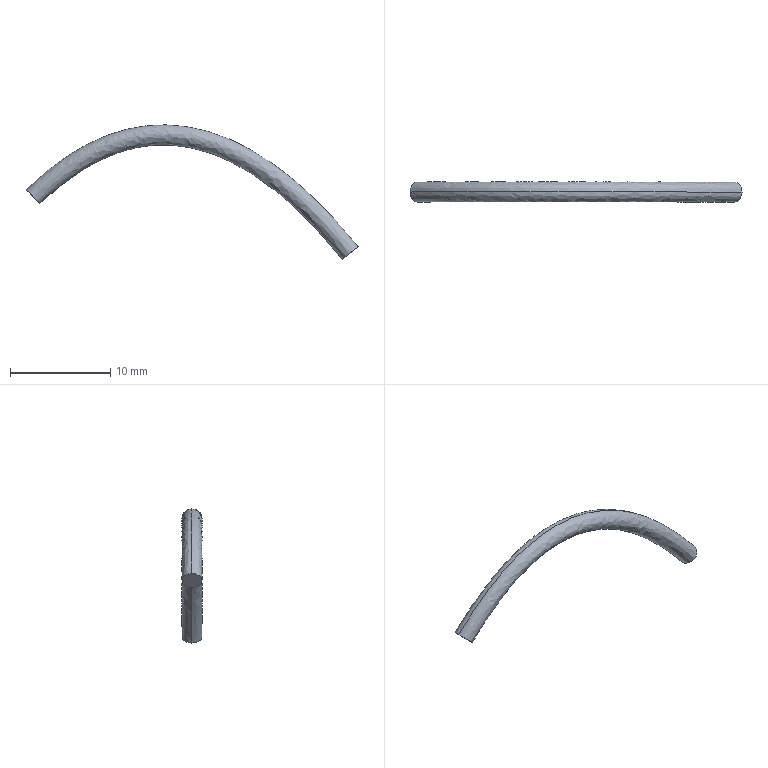Part | STEP file | YINGXIAN4_4_1 | 1 solid | 4 faces | box 33.17 x 2 x 13.408 mm | volume 118.062 mm3 | plane 2 | spline 2
STEP:
#1=CARTESIAN_POINT('',(0.,0.,0.));
#2=DIRECTION('',(0.,0.,1.));
#3=DIRECTION('',(1.,0.,0.));
#4=AXIS2_PLACEMENT_3D('',#1,#2,#3);
#5=CARTESIAN_POINT('',(0.6931,0.,-0.7208));
#6=VERTEX_POINT('',#5);
#7=CARTESIAN_POINT('',(-0.6931,0.,0.7208));
#8=VERTEX_POINT('',#7);
#9=CARTESIAN_POINT('',(0.6931,0.1194,-0.7208));
#10=CARTESIAN_POINT('',(0.6627,0.3767,-0.6892));
#11=CARTESIAN_POINT('',(0.5016,0.7326,-0.5216));
#12=CARTESIAN_POINT('',(0.2966,0.9207,-0.3085));
#13=CARTESIAN_POINT('',(0.1236,0.9898,-0.1286));
#14=CARTESIAN_POINT('',(0.,1.005,0.));
#15=CARTESIAN_POINT('',(-0.1236,0.9898,0.1286));
#16=CARTESIAN_POINT('',(-0.2966,0.9207,0.3085));
#17=CARTESIAN_POINT('',(-0.5016,0.7326,0.5216));
#18=CARTESIAN_POINT('',(-0.6627,0.3767,0.6892));
#19=CARTESIAN_POINT('',(-0.6931,0.1194,0.7208));
#20=B_SPLINE_CURVE_WITH_KNOTS('',3,(#5,#9,#10,#11,#12,#13,#14,#15,#16,#17,#18,#19,#7),.UNSPECIFIED.,.F.,.F.,(4,1,1,1,1,1,1,1,1,1,4),(0.,0.125,0.25,0.375,0.4375,0.5,0.5625,0.625,0.75,0.875,1.),.UNSPECIFIED.);
#21=EDGE_CURVE('',#6,#8,#20,.T.);
#22=ORIENTED_EDGE('',*,*,#21,.T.);
#23=CARTESIAN_POINT('',(-0.6931,0.,0.7208));
#24=CARTESIAN_POINT('',(-0.6931,-0.1194,0.7208));
#25=CARTESIAN_POINT('',(-0.6627,-0.3767,0.6892));
#26=CARTESIAN_POINT('',(-0.5016,-0.7326,0.5216));
#27=CARTESIAN_POINT('',(-0.2966,-0.9207,0.3085));
#28=CARTESIAN_POINT('',(-0.1236,-0.9898,0.1286));
#29=CARTESIAN_POINT('',(0.,-1.005,0.));
#30=CARTESIAN_POINT('',(0.1236,-0.9898,-0.1286));
#31=CARTESIAN_POINT('',(0.2966,-0.9207,-0.3085));
#32=CARTESIAN_POINT('',(0.5016,-0.7326,-0.5216));
#33=CARTESIAN_POINT('',(0.6627,-0.3767,-0.6892));
#34=CARTESIAN_POINT('',(0.6931,-0.1194,-0.7208));
#35=CARTESIAN_POINT('',(0.6931,0.,-0.7208));
#36=B_SPLINE_CURVE_WITH_KNOTS('',3,(#23,#24,#25,#26,#27,#28,#29,#30,#31,#32,#33,#34,#35),.UNSPECIFIED.,.F.,.F.,(4,1,1,1,1,1,1,1,1,1,4),(0.,0.125,0.25,0.375,0.4375,0.5,0.5625,0.625,0.75,0.875,1.),.UNSPECIFIED.);
#37=EDGE_CURVE('',#8,#6,#36,.T.);
#38=ORIENTED_EDGE('',*,*,#37,.T.);
#39=EDGE_LOOP('',(#22,#38));
#40=FACE_OUTER_BOUND('',#39,.F.);
#41=CARTESIAN_POINT('',(0.,0.,0.));
#42=DIRECTION('',(0.7208,0.,0.6931));
#43=DIRECTION('',(0.6931,0.,-0.7208));
#44=AXIS2_PLACEMENT_3D('',#41,#42,#43);
#45=PLANE('',#44);
#46=ADVANCED_FACE('',(#40),#45,.F.);
#47=ORIENTED_EDGE('',*,*,#21,.F.);
#48=CARTESIAN_POINT('',(30.923,0.,-6.249));
#49=VERTEX_POINT('',#48);
#50=CARTESIAN_POINT('',(0.6931,0.,-0.7208));
#51=CARTESIAN_POINT('',(2.159,0.,0.6885));
#52=CARTESIAN_POINT('',(4.382,0.,2.435));
#53=CARTESIAN_POINT('',(7.408,0.,4.024));
#54=CARTESIAN_POINT('',(9.717,0.,4.813));
#55=CARTESIAN_POINT('',(12.077,0.,5.194));
#56=CARTESIAN_POINT('',(14.439,0.,5.157));
#57=CARTESIAN_POINT('',(16.961,0.,4.657));
#58=CARTESIAN_POINT('',(20.428,0.,3.321));
#59=CARTESIAN_POINT('',(25.074,0.,0.2324));
#60=CARTESIAN_POINT('',(28.907,0.,-3.76));
#61=B_SPLINE_CURVE_WITH_KNOTS('',3,(#50,#51,#52,#53,#54,#55,#56,#57,#58,#59,#60,#48),.UNSPECIFIED.,.F.,.F.,(4,1,1,1,1,1,1,1,1,4),(0.,0.1483,0.2255,0.3091,0.3855,0.4682,0.551,0.6407,0.8132,1.),.UNSPECIFIED.);
#62=EDGE_CURVE('',#6,#49,#61,.T.);
#63=ORIENTED_EDGE('',*,*,#62,.T.);
#64=CARTESIAN_POINT('',(32.477,0.,-4.991));
#65=VERTEX_POINT('',#64);
#66=CARTESIAN_POINT('',(32.477,0.1194,-4.991));
#67=CARTESIAN_POINT('',(32.443,0.3767,-5.018));
#68=CARTESIAN_POINT('',(32.262,0.7326,-5.165));
#69=CARTESIAN_POINT('',(32.033,0.9207,-5.351));
#70=CARTESIAN_POINT('',(31.839,0.9898,-5.508));
#71=CARTESIAN_POINT('',(31.7,1.005,-5.62));
#72=CARTESIAN_POINT('',(31.561,0.9898,-5.732));
#73=CARTESIAN_POINT('',(31.367,0.9207,-5.889));
#74=CARTESIAN_POINT('',(31.138,0.7326,-6.075));
#75=CARTESIAN_POINT('',(30.957,0.3767,-6.222));
#76=CARTESIAN_POINT('',(30.923,0.1194,-6.249));
#77=CARTESIAN_POINT('',(30.923,0.,-6.249));
#78=B_SPLINE_CURVE_WITH_KNOTS('',3,(#64,#66,#67,#68,#69,#70,#71,#72,#73,#74,#75,#76,#77),.UNSPECIFIED.,.F.,.F.,(4,1,1,1,1,1,1,1,1,1,4),(0.,0.125,0.25,0.375,0.4375,0.5,0.5625,0.625,0.75,0.875,1.),.UNSPECIFIED.);
#79=EDGE_CURVE('',#65,#49,#78,.T.);
#80=ORIENTED_EDGE('',*,*,#79,.F.);
#81=CARTESIAN_POINT('',(-0.6931,0.,0.7208));
#82=CARTESIAN_POINT('',(0.8601,0.,2.214));
#83=CARTESIAN_POINT('',(3.251,0.,4.1));
#84=CARTESIAN_POINT('',(6.605,0.,5.865));
#85=CARTESIAN_POINT('',(9.22,0.,6.761));
#86=CARTESIAN_POINT('',(11.933,0.,7.2));
#87=CARTESIAN_POINT('',(14.657,0.,7.156));
#88=CARTESIAN_POINT('',(17.534,0.,6.584));
#89=CARTESIAN_POINT('',(21.407,0.,5.086));
#90=CARTESIAN_POINT('',(26.409,0.,1.742));
#91=CARTESIAN_POINT('',(30.398,0.,-2.424));
#92=CARTESIAN_POINT('',(32.477,0.,-4.991));
#93=B_SPLINE_CURVE_WITH_KNOTS('',3,(#81,#82,#83,#84,#85,#86,#87,#88,#89,#90,#91,#92),.UNSPECIFIED.,.F.,.F.,(4,1,1,1,1,1,1,1,1,4),(0.,0.1483,0.2255,0.3091,0.3855,0.4682,0.551,0.6407,0.8132,1.),.UNSPECIFIED.);
#94=EDGE_CURVE('',#8,#65,#93,.T.);
#95=ORIENTED_EDGE('',*,*,#94,.F.);
#96=EDGE_LOOP('',(#47,#63,#80,#95));
#97=FACE_OUTER_BOUND('',#96,.F.);
#98=CARTESIAN_POINT('',(0.4367,-0.03181,-0.9693));
#99=CARTESIAN_POINT('',(1.988,-0.03181,0.5542));
#100=CARTESIAN_POINT('',(4.298,-0.03181,2.391));
#101=CARTESIAN_POINT('',(7.408,-0.03181,4.025));
#102=CARTESIAN_POINT('',(9.717,-0.03181,4.814));
#103=CARTESIAN_POINT('',(12.077,-0.03181,5.195));
#104=CARTESIAN_POINT('',(14.439,-0.03181,5.157));
#105=CARTESIAN_POINT('',(16.961,-0.03181,4.658));
#106=CARTESIAN_POINT('',(20.429,-0.03181,3.321));
#107=CARTESIAN_POINT('',(25.147,-0.03181,0.1847));
#108=CARTESIAN_POINT('',(29.057,-0.03181,-3.916));
#109=CARTESIAN_POINT('',(31.15,-0.03181,-6.53));
#110=CARTESIAN_POINT('',(0.4397,0.09633,-0.9723));
#111=CARTESIAN_POINT('',(1.991,0.09633,0.551));
#112=CARTESIAN_POINT('',(4.3,0.09633,2.388));
#113=CARTESIAN_POINT('',(7.41,0.09633,4.021));
#114=CARTESIAN_POINT('',(9.718,0.09633,4.81));
#115=CARTESIAN_POINT('',(12.077,0.09633,5.19));
#116=CARTESIAN_POINT('',(14.439,0.09633,5.153));
#117=CARTESIAN_POINT('',(16.959,0.09633,4.654));
#118=CARTESIAN_POINT('',(20.427,0.09633,3.317));
#119=CARTESIAN_POINT('',(25.144,0.09633,0.1816));
#120=CARTESIAN_POINT('',(29.054,0.09633,-3.919));
#121=CARTESIAN_POINT('',(31.146,0.09633,-6.533));
#122=CARTESIAN_POINT('',(0.4112,0.3661,-0.9433));
#123=CARTESIAN_POINT('',(1.964,0.3661,0.5818));
#124=CARTESIAN_POINT('',(4.277,0.3661,2.422));
#125=CARTESIAN_POINT('',(7.393,0.3661,4.058));
#126=CARTESIAN_POINT('',(9.708,0.3661,4.849));
#127=CARTESIAN_POINT('',(12.074,0.3661,5.231));
#128=CARTESIAN_POINT('',(14.443,0.3661,5.194));
#129=CARTESIAN_POINT('',(16.971,0.3661,4.693));
#130=CARTESIAN_POINT('',(20.447,0.3661,3.353));
#131=CARTESIAN_POINT('',(25.171,0.3661,0.2122));
#132=CARTESIAN_POINT('',(29.084,0.3661,-3.892));
#133=CARTESIAN_POINT('',(31.178,0.3661,-6.507));
#134=CARTESIAN_POINT('',(0.2435,0.7326,-0.7725));
#135=CARTESIAN_POINT('',(1.807,0.7326,0.7631));
#136=CARTESIAN_POINT('',(4.14,0.7326,2.62));
#137=CARTESIAN_POINT('',(7.297,0.7326,4.279));
#138=CARTESIAN_POINT('',(9.649,0.7326,5.082));
#139=CARTESIAN_POINT('',(12.057,0.7326,5.471));
#140=CARTESIAN_POINT('',(14.469,0.7326,5.433));
#141=CARTESIAN_POINT('',(17.04,0.7326,4.923));
#142=CARTESIAN_POINT('',(20.564,0.7326,3.565));
#143=CARTESIAN_POINT('',(25.331,0.7326,0.3923));
#144=CARTESIAN_POINT('',(29.263,0.7326,-3.733));
#145=CARTESIAN_POINT('',(31.365,0.7326,-6.358));
#146=CARTESIAN_POINT('',(0.03628,0.9207,-0.5615));
#147=CARTESIAN_POINT('',(1.613,0.9207,0.9871));
#148=CARTESIAN_POINT('',(3.972,0.9207,2.866));
#149=CARTESIAN_POINT('',(7.178,0.9207,4.551));
#150=CARTESIAN_POINT('',(9.575,0.9207,5.37));
#151=CARTESIAN_POINT('',(12.036,0.9207,5.768));
#152=CARTESIAN_POINT('',(14.501,0.9207,5.728));
#153=CARTESIAN_POINT('',(17.124,0.9207,5.208));
#154=CARTESIAN_POINT('',(20.708,0.9207,3.826));
#155=CARTESIAN_POINT('',(25.53,0.9207,0.6148));
#156=CARTESIAN_POINT('',(29.484,0.9207,-3.536));
#157=CARTESIAN_POINT('',(31.596,0.9207,-6.173));
#158=CARTESIAN_POINT('',(-0.1386,0.9898,-0.3834));
#159=CARTESIAN_POINT('',(1.45,0.9897,1.176));
#160=CARTESIAN_POINT('',(3.829,0.9898,3.073));
#161=CARTESIAN_POINT('',(7.078,0.9898,4.78));
#162=CARTESIAN_POINT('',(9.513,0.9898,5.613));
#163=CARTESIAN_POINT('',(12.018,0.9898,6.018));
#164=CARTESIAN_POINT('',(14.529,0.9897,5.978));
#165=CARTESIAN_POINT('',(17.196,0.9897,5.449));
#166=CARTESIAN_POINT('',(20.83,0.9898,4.046));
#167=CARTESIAN_POINT('',(25.697,0.9898,0.8026));
#168=CARTESIAN_POINT('',(29.671,0.9897,-3.37));
#169=CARTESIAN_POINT('',(31.791,0.9898,-6.017));
#170=CARTESIAN_POINT('',(-0.2636,1.005,-0.2562));
#171=CARTESIAN_POINT('',(1.333,1.005,1.311));
#172=CARTESIAN_POINT('',(3.728,1.005,3.221));
#173=CARTESIAN_POINT('',(7.007,1.005,4.945));
#174=CARTESIAN_POINT('',(9.469,1.005,5.787));
#175=CARTESIAN_POINT('',(12.005,1.005,6.197));
#176=CARTESIAN_POINT('',(14.548,1.005,6.156));
#177=CARTESIAN_POINT('',(17.247,1.005,5.621));
#178=CARTESIAN_POINT('',(20.918,1.005,4.204));
#179=CARTESIAN_POINT('',(25.817,1.005,0.9369));
#180=CARTESIAN_POINT('',(29.805,1.005,-3.251));
#181=CARTESIAN_POINT('',(31.93,1.005,-5.905));
#182=CARTESIAN_POINT('',(-0.3886,0.9898,-0.1289));
#183=CARTESIAN_POINT('',(1.216,0.9897,1.447));
#184=CARTESIAN_POINT('',(3.626,0.9898,3.369));
#185=CARTESIAN_POINT('',(6.935,0.9898,5.109));
#186=CARTESIAN_POINT('',(9.425,0.9898,5.961));
#187=CARTESIAN_POINT('',(11.992,0.9898,6.376));
#188=CARTESIAN_POINT('',(14.568,0.9897,6.334));
#189=CARTESIAN_POINT('',(17.298,0.9897,5.793));
#190=CARTESIAN_POINT('',(21.005,0.9898,4.361));
#191=CARTESIAN_POINT('',(25.936,0.9898,1.071));
#192=CARTESIAN_POINT('',(29.938,0.9897,-3.133));
#193=CARTESIAN_POINT('',(32.069,0.9898,-5.794));
#194=CARTESIAN_POINT('',(-0.5635,0.9207,0.0492));
#195=CARTESIAN_POINT('',(1.052,0.9207,1.636));
#196=CARTESIAN_POINT('',(3.484,0.9207,3.576));
#197=CARTESIAN_POINT('',(6.835,0.9207,5.338));
#198=CARTESIAN_POINT('',(9.363,0.9207,6.204));
#199=CARTESIAN_POINT('',(11.974,0.9207,6.626));
#200=CARTESIAN_POINT('',(14.595,0.9207,6.584));
#201=CARTESIAN_POINT('',(17.37,0.9207,6.033));
#202=CARTESIAN_POINT('',(21.127,0.9207,4.581));
#203=CARTESIAN_POINT('',(26.104,0.9207,1.259));
#204=CARTESIAN_POINT('',(30.125,0.9207,-2.967));
#205=CARTESIAN_POINT('',(32.264,0.9207,-5.638));
#206=CARTESIAN_POINT('',(-0.7707,0.7326,0.2602));
#207=CARTESIAN_POINT('',(0.8581,0.7326,1.86));
#208=CARTESIAN_POINT('',(3.315,0.7326,3.821));
#209=CARTESIAN_POINT('',(6.716,0.7326,5.611));
#210=CARTESIAN_POINT('',(9.289,0.7326,6.492));
#211=CARTESIAN_POINT('',(11.953,0.7326,6.922));
#212=CARTESIAN_POINT('',(14.627,0.7326,6.88));
#213=CARTESIAN_POINT('',(17.454,0.7326,6.318));
#214=CARTESIAN_POINT('',(21.272,0.7326,4.842));
#215=CARTESIAN_POINT('',(26.302,0.7326,1.482));
#216=CARTESIAN_POINT('',(30.346,0.7326,-2.77));
#217=CARTESIAN_POINT('',(32.495,0.7326,-5.453));
#218=CARTESIAN_POINT('',(-0.9383,0.3663,0.4309));
#219=CARTESIAN_POINT('',(0.7012,0.3663,2.041));
#220=CARTESIAN_POINT('',(3.178,0.3663,4.02));
#221=CARTESIAN_POINT('',(6.62,0.3663,5.831));
#222=CARTESIAN_POINT('',(9.23,0.3663,6.725));
#223=CARTESIAN_POINT('',(11.936,0.3663,7.162));
#224=CARTESIAN_POINT('',(14.653,0.3663,7.119));
#225=CARTESIAN_POINT('',(17.523,0.3663,6.548));
#226=CARTESIAN_POINT('',(21.389,0.3663,5.054));
#227=CARTESIAN_POINT('',(26.462,0.3663,1.662));
#228=CARTESIAN_POINT('',(30.525,0.3663,-2.611));
#229=CARTESIAN_POINT('',(32.682,0.3663,-5.304));
#230=CARTESIAN_POINT('',(-0.9668,0.09668,0.4599));
#231=CARTESIAN_POINT('',(0.6746,0.09668,2.072));
#232=CARTESIAN_POINT('',(3.155,0.09668,4.054));
#233=CARTESIAN_POINT('',(6.604,0.09668,5.868));
#234=CARTESIAN_POINT('',(9.22,0.09668,6.764));
#235=CARTESIAN_POINT('',(11.933,0.09668,7.203));
#236=CARTESIAN_POINT('',(14.658,0.09668,7.159));
#237=CARTESIAN_POINT('',(17.535,0.09668,6.588));
#238=CARTESIAN_POINT('',(21.409,0.09668,5.09));
#239=CARTESIAN_POINT('',(26.49,0.09668,1.692));
#240=CARTESIAN_POINT('',(30.556,0.09668,-2.584));
#241=CARTESIAN_POINT('',(32.713,0.09668,-5.278));
#242=CARTESIAN_POINT('',(-0.9639,-0.03133,0.457));
#243=CARTESIAN_POINT('',(0.6773,-0.03133,2.069));
#244=CARTESIAN_POINT('',(3.158,-0.03133,4.05));
#245=CARTESIAN_POINT('',(6.605,-0.03133,5.864));
#246=CARTESIAN_POINT('',(9.221,-0.03133,6.76));
#247=CARTESIAN_POINT('',(11.933,-0.03133,7.199));
#248=CARTESIAN_POINT('',(14.657,-0.03133,7.155));
#249=CARTESIAN_POINT('',(17.533,-0.03133,6.584));
#250=CARTESIAN_POINT('',(21.407,-0.03133,5.086));
#251=CARTESIAN_POINT('',(26.487,-0.03133,1.689));
#252=CARTESIAN_POINT('',(30.553,-0.03133,-2.586));
#253=CARTESIAN_POINT('',(32.71,-0.03133,-5.281));
#254=B_SPLINE_SURFACE_WITH_KNOTS('',3,3,((#98,#99,#100,#101,#102,#103,#104,#105,#106,#107,#108,#109),(#110,#111,#112,#113,#114,#115,#116,#117,#118,#119,#120,#121),(#122,#123,#124,#125,#126,#127,#128,#129,#130,#131,#132,#133),(#134,#135,#136,#137,#138,#139,#140,#141,#142,#143,#144,#145),(#146,#147,#148,#149,#150,#151,#152,#153,#154,#155,#156,#157),(#158,#159,#160,#161,#162,#163,#164,#165,#166,#167,#168,#169),(#170,#171,#172,#173,#174,#175,#176,#177,#178,#179,#180,#181),(#182,#183,#184,#185,#186,#187,#188,#189,#190,#191,#192,#193),(#194,#195,#196,#197,#198,#199,#200,#201,#202,#203,#204,#205),(#206,#207,#208,#209,#210,#211,#212,#213,#214,#215,#216,#217),(#218,#219,#220,#221,#222,#223,#224,#225,#226,#227,#228,#229),(#230,#231,#232,#233,#234,#235,#236,#237,#238,#239,#240,#241),(#242,#243,#244,#245,#246,#247,#248,#249,#250,#251,#252,#253)),.UNSPECIFIED.,.F.,.F.,.F.,(4,1,1,1,1,1,1,1,1,1,4),(4,1,1,1,1,1,1,1,1,4),(0.02112,0.2819,0.5213,0.7606,0.8803,1.,1.12,1.239,1.479,1.718,1.979),(-0.008638,0.1483,0.2255,0.3091,0.3855,0.4682,0.551,0.6407,0.8132,1.007),.UNSPECIFIED.);
#255=ADVANCED_FACE('',(#97),#254,.T.);
#256=ORIENTED_EDGE('',*,*,#37,.F.);
#257=ORIENTED_EDGE('',*,*,#94,.T.);
#258=CARTESIAN_POINT('',(30.923,0.,-6.249));
#259=CARTESIAN_POINT('',(30.923,-0.1194,-6.249));
#260=CARTESIAN_POINT('',(30.957,-0.3767,-6.222));
#261=CARTESIAN_POINT('',(31.138,-0.7326,-6.075));
#262=CARTESIAN_POINT('',(31.367,-0.9207,-5.889));
#263=CARTESIAN_POINT('',(31.561,-0.9898,-5.732));
#264=CARTESIAN_POINT('',(31.7,-1.005,-5.62));
#265=CARTESIAN_POINT('',(31.839,-0.9898,-5.508));
#266=CARTESIAN_POINT('',(32.033,-0.9207,-5.351));
#267=CARTESIAN_POINT('',(32.262,-0.7326,-5.165));
#268=CARTESIAN_POINT('',(32.443,-0.3767,-5.018));
#269=CARTESIAN_POINT('',(32.477,-0.1194,-4.991));
#270=CARTESIAN_POINT('',(32.477,0.,-4.991));
#271=B_SPLINE_CURVE_WITH_KNOTS('',3,(#258,#259,#260,#261,#262,#263,#264,#265,#266,#267,#268,#269,#270),.UNSPECIFIED.,.F.,.F.,(4,1,1,1,1,1,1,1,1,1,4),(0.,0.125,0.25,0.375,0.4375,0.5,0.5625,0.625,0.75,0.875,1.),.UNSPECIFIED.);
#272=EDGE_CURVE('',#49,#65,#271,.T.);
#273=ORIENTED_EDGE('',*,*,#272,.F.);
#274=ORIENTED_EDGE('',*,*,#62,.F.);
#275=EDGE_LOOP('',(#256,#257,#273,#274));
#276=FACE_OUTER_BOUND('',#275,.F.);
#277=CARTESIAN_POINT('',(-0.9639,0.03181,0.4569));
#278=CARTESIAN_POINT('',(0.6773,0.03181,2.069));
#279=CARTESIAN_POINT('',(3.158,0.03181,4.05));
#280=CARTESIAN_POINT('',(6.605,0.03181,5.864));
#281=CARTESIAN_POINT('',(9.221,0.03181,6.76));
#282=CARTESIAN_POINT('',(11.933,0.03181,7.199));
#283=CARTESIAN_POINT('',(14.657,0.03181,7.155));
#284=CARTESIAN_POINT('',(17.533,0.03181,6.584));
#285=CARTESIAN_POINT('',(21.407,0.03181,5.086));
#286=CARTESIAN_POINT('',(26.487,0.03181,1.689));
#287=CARTESIAN_POINT('',(30.553,0.03181,-2.587));
#288=CARTESIAN_POINT('',(32.71,0.03181,-5.281));
#289=CARTESIAN_POINT('',(-0.9669,-0.09633,0.46));
#290=CARTESIAN_POINT('',(0.6745,-0.09633,2.072));
#291=CARTESIAN_POINT('',(3.155,-0.09633,4.054));
#292=CARTESIAN_POINT('',(6.604,-0.09633,5.868));
#293=CARTESIAN_POINT('',(9.22,-0.09633,6.764));
#294=CARTESIAN_POINT('',(11.933,-0.09633,7.203));
#295=CARTESIAN_POINT('',(14.658,-0.09633,7.159));
#296=CARTESIAN_POINT('',(17.535,-0.09633,6.588));
#297=CARTESIAN_POINT('',(21.409,-0.09633,5.09));
#298=CARTESIAN_POINT('',(26.49,-0.09633,1.692));
#299=CARTESIAN_POINT('',(30.556,-0.09633,-2.584));
#300=CARTESIAN_POINT('',(32.713,-0.09633,-5.278));
#301=CARTESIAN_POINT('',(-0.9384,-0.3661,0.431));
#302=CARTESIAN_POINT('',(0.7012,-0.3661,2.041));
#303=CARTESIAN_POINT('',(3.178,-0.3661,4.02));
#304=CARTESIAN_POINT('',(6.62,-0.3661,5.831));
#305=CARTESIAN_POINT('',(9.23,-0.3661,6.725));
#306=CARTESIAN_POINT('',(11.936,-0.3661,7.162));
#307=CARTESIAN_POINT('',(14.653,-0.3661,7.119));
#308=CARTESIAN_POINT('',(17.523,-0.3661,6.548));
#309=CARTESIAN_POINT('',(21.389,-0.3661,5.054));
#310=CARTESIAN_POINT('',(26.462,-0.3661,1.662));
#311=CARTESIAN_POINT('',(30.526,-0.3661,-2.611));
#312=CARTESIAN_POINT('',(32.682,-0.3661,-5.304));
#313=CARTESIAN_POINT('',(-0.7707,-0.7326,0.2602));
#314=CARTESIAN_POINT('',(0.8581,-0.7326,1.86));
#315=CARTESIAN_POINT('',(3.315,-0.7326,3.821));
#316=CARTESIAN_POINT('',(6.716,-0.7326,5.611));
#317=CARTESIAN_POINT('',(9.289,-0.7326,6.492));
#318=CARTESIAN_POINT('',(11.953,-0.7326,6.922));
#319=CARTESIAN_POINT('',(14.627,-0.7326,6.88));
#320=CARTESIAN_POINT('',(17.454,-0.7326,6.318));
#321=CARTESIAN_POINT('',(21.272,-0.7326,4.842));
#322=CARTESIAN_POINT('',(26.302,-0.7326,1.482));
#323=CARTESIAN_POINT('',(30.346,-0.7326,-2.77));
#324=CARTESIAN_POINT('',(32.495,-0.7326,-5.453));
#325=CARTESIAN_POINT('',(-0.5635,-0.9207,0.0492));
#326=CARTESIAN_POINT('',(1.052,-0.9207,1.636));
#327=CARTESIAN_POINT('',(3.484,-0.9207,3.576));
#328=CARTESIAN_POINT('',(6.835,-0.9207,5.338));
#329=CARTESIAN_POINT('',(9.363,-0.9207,6.204));
#330=CARTESIAN_POINT('',(11.974,-0.9207,6.626));
#331=CARTESIAN_POINT('',(14.595,-0.9207,6.584));
#332=CARTESIAN_POINT('',(17.37,-0.9207,6.033));
#333=CARTESIAN_POINT('',(21.127,-0.9207,4.581));
#334=CARTESIAN_POINT('',(26.104,-0.9207,1.259));
#335=CARTESIAN_POINT('',(30.125,-0.9207,-2.967));
#336=CARTESIAN_POINT('',(32.264,-0.9207,-5.638));
#337=CARTESIAN_POINT('',(-0.3886,-0.9898,-0.1289));
#338=CARTESIAN_POINT('',(1.216,-0.9897,1.447));
#339=CARTESIAN_POINT('',(3.626,-0.9898,3.369));
#340=CARTESIAN_POINT('',(6.935,-0.9898,5.109));
#341=CARTESIAN_POINT('',(9.425,-0.9898,5.961));
#342=CARTESIAN_POINT('',(11.992,-0.9898,6.376));
#343=CARTESIAN_POINT('',(14.568,-0.9897,6.334));
#344=CARTESIAN_POINT('',(17.298,-0.9897,5.793));
#345=CARTESIAN_POINT('',(21.005,-0.9898,4.361));
#346=CARTESIAN_POINT('',(25.936,-0.9898,1.071));
#347=CARTESIAN_POINT('',(29.938,-0.9897,-3.133));
#348=CARTESIAN_POINT('',(32.069,-0.9898,-5.794));
#349=CARTESIAN_POINT('',(-0.2636,-1.005,-0.2562));
#350=CARTESIAN_POINT('',(1.333,-1.005,1.311));
#351=CARTESIAN_POINT('',(3.728,-1.005,3.221));
#352=CARTESIAN_POINT('',(7.007,-1.005,4.945));
#353=CARTESIAN_POINT('',(9.469,-1.005,5.787));
#354=CARTESIAN_POINT('',(12.005,-1.005,6.197));
#355=CARTESIAN_POINT('',(14.548,-1.005,6.156));
#356=CARTESIAN_POINT('',(17.247,-1.005,5.621));
#357=CARTESIAN_POINT('',(20.918,-1.005,4.204));
#358=CARTESIAN_POINT('',(25.817,-1.005,0.9369));
#359=CARTESIAN_POINT('',(29.805,-1.005,-3.251));
#360=CARTESIAN_POINT('',(31.93,-1.005,-5.905));
#361=CARTESIAN_POINT('',(-0.1386,-0.9898,-0.3834));
#362=CARTESIAN_POINT('',(1.45,-0.9897,1.176));
#363=CARTESIAN_POINT('',(3.829,-0.9898,3.073));
#364=CARTESIAN_POINT('',(7.078,-0.9898,4.78));
#365=CARTESIAN_POINT('',(9.513,-0.9898,5.613));
#366=CARTESIAN_POINT('',(12.018,-0.9898,6.018));
#367=CARTESIAN_POINT('',(14.529,-0.9897,5.978));
#368=CARTESIAN_POINT('',(17.196,-0.9897,5.449));
#369=CARTESIAN_POINT('',(20.83,-0.9898,4.046));
#370=CARTESIAN_POINT('',(25.697,-0.9898,0.8026));
#371=CARTESIAN_POINT('',(29.671,-0.9897,-3.37));
#372=CARTESIAN_POINT('',(31.791,-0.9898,-6.017));
#373=CARTESIAN_POINT('',(0.03628,-0.9207,-0.5615));
#374=CARTESIAN_POINT('',(1.613,-0.9207,0.9871));
#375=CARTESIAN_POINT('',(3.972,-0.9207,2.866));
#376=CARTESIAN_POINT('',(7.178,-0.9207,4.551));
#377=CARTESIAN_POINT('',(9.575,-0.9207,5.37));
#378=CARTESIAN_POINT('',(12.036,-0.9207,5.768));
#379=CARTESIAN_POINT('',(14.501,-0.9207,5.728));
#380=CARTESIAN_POINT('',(17.124,-0.9207,5.208));
#381=CARTESIAN_POINT('',(20.708,-0.9207,3.826));
#382=CARTESIAN_POINT('',(25.53,-0.9207,0.6148));
#383=CARTESIAN_POINT('',(29.484,-0.9207,-3.536));
#384=CARTESIAN_POINT('',(31.596,-0.9207,-6.173));
#385=CARTESIAN_POINT('',(0.2435,-0.7326,-0.7725));
#386=CARTESIAN_POINT('',(1.807,-0.7326,0.7631));
#387=CARTESIAN_POINT('',(4.14,-0.7326,2.62));
#388=CARTESIAN_POINT('',(7.297,-0.7326,4.279));
#389=CARTESIAN_POINT('',(9.649,-0.7326,5.082));
#390=CARTESIAN_POINT('',(12.057,-0.7326,5.471));
#391=CARTESIAN_POINT('',(14.469,-0.7326,5.433));
#392=CARTESIAN_POINT('',(17.04,-0.7326,4.923));
#393=CARTESIAN_POINT('',(20.564,-0.7326,3.565));
#394=CARTESIAN_POINT('',(25.331,-0.7326,0.3923));
#395=CARTESIAN_POINT('',(29.263,-0.7326,-3.733));
#396=CARTESIAN_POINT('',(31.365,-0.7326,-6.358));
#397=CARTESIAN_POINT('',(0.4111,-0.3663,-0.9432));
#398=CARTESIAN_POINT('',(1.964,-0.3663,0.5819));
#399=CARTESIAN_POINT('',(4.277,-0.3663,2.422));
#400=CARTESIAN_POINT('',(7.393,-0.3663,4.059));
#401=CARTESIAN_POINT('',(9.708,-0.3663,4.849));
#402=CARTESIAN_POINT('',(12.074,-0.3663,5.231));
#403=CARTESIAN_POINT('',(14.443,-0.3663,5.194));
#404=CARTESIAN_POINT('',(16.971,-0.3663,4.693));
#405=CARTESIAN_POINT('',(20.447,-0.3663,3.353));
#406=CARTESIAN_POINT('',(25.171,-0.3663,0.2122));
#407=CARTESIAN_POINT('',(29.084,-0.3663,-3.892));
#408=CARTESIAN_POINT('',(31.178,-0.3663,-6.507));
#409=CARTESIAN_POINT('',(0.4396,-0.09668,-0.9723));
#410=CARTESIAN_POINT('',(1.991,-0.09668,0.551));
#411=CARTESIAN_POINT('',(4.3,-0.09668,2.388));
#412=CARTESIAN_POINT('',(7.41,-0.09668,4.021));
#413=CARTESIAN_POINT('',(9.718,-0.09668,4.81));
#414=CARTESIAN_POINT('',(12.077,-0.09668,5.19));
#415=CARTESIAN_POINT('',(14.439,-0.09668,5.153));
#416=CARTESIAN_POINT('',(16.959,-0.09668,4.654));
#417=CARTESIAN_POINT('',(20.427,-0.09668,3.318));
#418=CARTESIAN_POINT('',(25.144,-0.09668,0.1816));
#419=CARTESIAN_POINT('',(29.054,-0.09668,-3.919));
#420=CARTESIAN_POINT('',(31.146,-0.09668,-6.533));
#421=CARTESIAN_POINT('',(0.4367,0.03133,-0.9693));
#422=CARTESIAN_POINT('',(1.988,0.03133,0.5542));
#423=CARTESIAN_POINT('',(4.298,0.03133,2.391));
#424=CARTESIAN_POINT('',(7.408,0.03133,4.025));
#425=CARTESIAN_POINT('',(9.717,0.03133,4.814));
#426=CARTESIAN_POINT('',(12.077,0.03133,5.195));
#427=CARTESIAN_POINT('',(14.439,0.03133,5.157));
#428=CARTESIAN_POINT('',(16.961,0.03133,4.658));
#429=CARTESIAN_POINT('',(20.429,0.03133,3.321));
#430=CARTESIAN_POINT('',(25.147,0.03133,0.1847));
#431=CARTESIAN_POINT('',(29.057,0.03133,-3.916));
#432=CARTESIAN_POINT('',(31.15,0.03133,-6.53));
#433=B_SPLINE_SURFACE_WITH_KNOTS('',3,3,((#277,#278,#279,#280,#281,#282,#283,#284,#285,#286,#287,#288),(#289,#290,#291,#292,#293,#294,#295,#296,#297,#298,#299,#300),(#301,#302,#303,#304,#305,#306,#307,#308,#309,#310,#311,#312),(#313,#314,#315,#316,#317,#318,#319,#320,#321,#322,#323,#324),(#325,#326,#327,#328,#329,#330,#331,#332,#333,#334,#335,#336),(#337,#338,#339,#340,#341,#342,#343,#344,#345,#346,#347,#348),(#349,#350,#351,#352,#353,#354,#355,#356,#357,#358,#359,#360),(#361,#362,#363,#364,#365,#366,#367,#368,#369,#370,#371,#372),(#373,#374,#375,#376,#377,#378,#379,#380,#381,#382,#383,#384),(#385,#386,#387,#388,#389,#390,#391,#392,#393,#394,#395,#396),(#397,#398,#399,#400,#401,#402,#403,#404,#405,#406,#407,#408),(#409,#410,#411,#412,#413,#414,#415,#416,#417,#418,#419,#420),(#421,#422,#423,#424,#425,#426,#427,#428,#429,#430,#431,#432)),.UNSPECIFIED.,.F.,.F.,.F.,(4,1,1,1,1,1,1,1,1,1,4),(4,1,1,1,1,1,1,1,1,4),(0.02112,0.2819,0.5213,0.7606,0.8803,1.,1.12,1.239,1.479,1.718,1.979),(-0.008638,0.1483,0.2255,0.3091,0.3855,0.4682,0.551,0.6407,0.8132,1.007),.UNSPECIFIED.);
#434=ADVANCED_FACE('',(#276),#433,.T.);
#435=ORIENTED_EDGE('',*,*,#79,.T.);
#436=ORIENTED_EDGE('',*,*,#272,.T.);
#437=EDGE_LOOP('',(#435,#436));
#438=FACE_OUTER_BOUND('',#437,.F.);
#439=CARTESIAN_POINT('',(31.7,0.,-5.62));
#440=DIRECTION('',(0.6294,0.,-0.7771));
#441=DIRECTION('',(-0.7771,0.,-0.6294));
#442=AXIS2_PLACEMENT_3D('',#439,#440,#441);
#443=PLANE('',#442);
#444=ADVANCED_FACE('',(#438),#443,.T.);
#445=CLOSED_SHELL('',(#46,#255,#434,#444));
#446=MANIFOLD_SOLID_BREP('',#445);
#447=(LENGTH_UNIT()NAMED_UNIT(*)SI_UNIT(.MILLI.,.METRE.));
#448=UNCERTAINTY_MEASURE_WITH_UNIT(LENGTH_MEASURE(0.003595),#447,'','');
#449=(NAMED_UNIT(*)PLANE_ANGLE_UNIT()SI_UNIT($,.RADIAN.));
#450=PLANE_ANGLE_MEASURE_WITH_UNIT(PLANE_ANGLE_MEASURE(0.01745),#449);
#451=(CONVERSION_BASED_UNIT('DEGREE',#450)NAMED_UNIT(*)PLANE_ANGLE_UNIT());
#452=(NAMED_UNIT(*)SI_UNIT($,.STERADIAN.)SOLID_ANGLE_UNIT());
#453=(GEOMETRIC_REPRESENTATION_CONTEXT(3)GLOBAL_UNCERTAINTY_ASSIGNED_CONTEXT((#448))GLOBAL_UNIT_ASSIGNED_CONTEXT((#447,#451,#452))REPRESENTATION_CONTEXT('',''));
#454=ADVANCED_BREP_SHAPE_REPRESENTATION('',(#4,#446),#453);